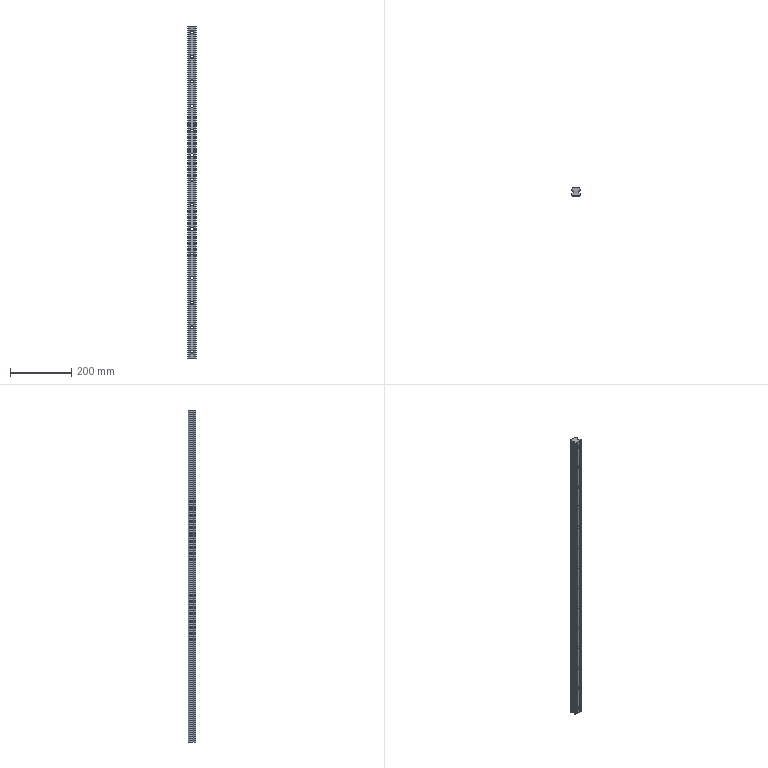Part | SolidWorks | features BaseBody 1 | 1 solid | 122 faces | box 28 x 26 x 1080 mm | volume 623982 mm3 | cylinder 78 | plane 44 | commonest cylinder face diameters 9 x28 14 x28 1.2 x12 1.6 x6 5.66 x4